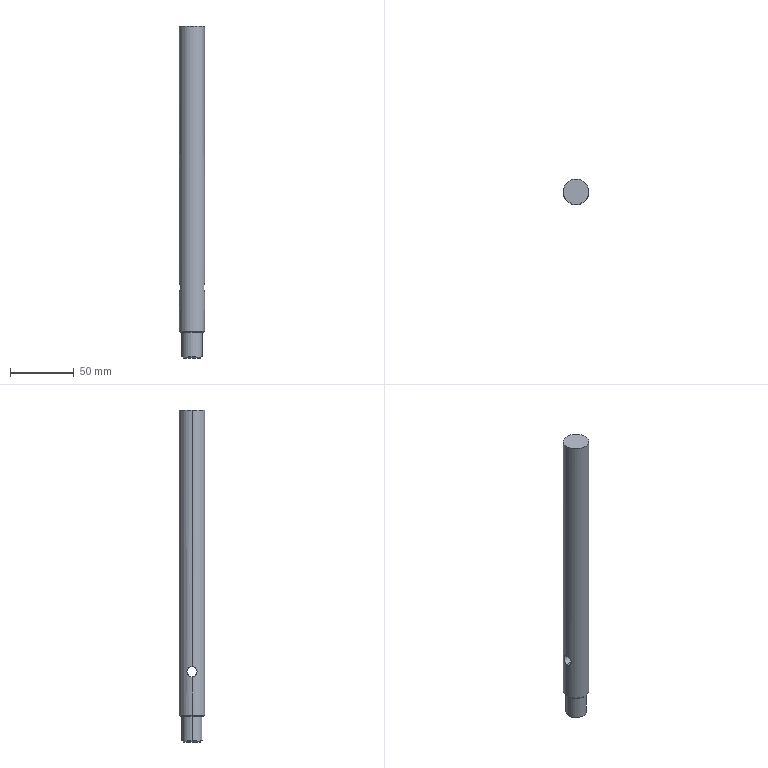Part | SolidWorks | features ICE 4, Chamfer 2, Revolution 1 | 1 solid | 13 faces | box 20 x 20 x 260 mm | volume 78380 mm3 | cylinder 6 | cone 4 | plane 3 | commonest cylinder face diameters 8 x2 16 x2 20 x2
STEP:
#1=CARTESIAN_POINT('',(-9.,0.,-170.));
#2=VERTEX_POINT('',#1);
#3=CARTESIAN_POINT('',(9.,0.,-170.));
#4=VERTEX_POINT('',#3);
#5=CARTESIAN_POINT('',(0.,0.,-170.));
#6=DIRECTION('',(0.,0.,-1.));
#7=DIRECTION('',(-1.,0.,0.));
#8=AXIS2_PLACEMENT_3D('',#5,#6,#7);
#9=CIRCLE('',#8,9.);
#10=EDGE_CURVE('',#2,#4,#9,.T.);
#11=ORIENTED_EDGE('',*,*,#10,.F.);
#12=CARTESIAN_POINT('',(-10.,0.,-169.));
#13=VERTEX_POINT('',#12);
#14=CARTESIAN_POINT('',(-9.,0.,-170.));
#15=DIRECTION('',(-0.7071,0.,0.7071));
#16=VECTOR('',#15,1000.);
#17=LINE('',#14,#16);
#18=EDGE_CURVE('',#2,#13,#17,.T.);
#19=ORIENTED_EDGE('',*,*,#18,.T.);
#20=CARTESIAN_POINT('',(10.,0.,-169.));
#21=VERTEX_POINT('',#20);
#22=CARTESIAN_POINT('',(0.,0.,-169.));
#23=DIRECTION('',(0.,0.,1.));
#24=DIRECTION('',(-1.,0.,0.));
#25=AXIS2_PLACEMENT_3D('',#22,#23,#24);
#26=CIRCLE('',#25,10.);
#27=EDGE_CURVE('',#21,#13,#26,.T.);
#28=ORIENTED_EDGE('',*,*,#27,.F.);
#29=CARTESIAN_POINT('',(9.,0.,-170.));
#30=DIRECTION('',(0.7071,0.,0.7071));
#31=VECTOR('',#30,1000.);
#32=LINE('',#29,#31);
#33=EDGE_CURVE('',#4,#21,#32,.T.);
#34=ORIENTED_EDGE('',*,*,#33,.F.);
#35=EDGE_LOOP('',(#11,#19,#28,#34));
#36=FACE_OUTER_BOUND('',#35,.T.);
#37=CARTESIAN_POINT('',(0.,0.,-170.));
#38=DIRECTION('',(0.,0.,1.));
#39=DIRECTION('',(1.,0.,0.));
#40=AXIS2_PLACEMENT_3D('',#37,#38,#39);
#41=CONICAL_SURFACE('',#40,9.,0.7854);
#42=ADVANCED_FACE('',(#36),#41,.T.);
#43=CARTESIAN_POINT('',(-7.,0.,-190.));
#44=VERTEX_POINT('',#43);
#45=CARTESIAN_POINT('',(7.,0.,-190.));
#46=VERTEX_POINT('',#45);
#47=CARTESIAN_POINT('',(0.,0.,-190.));
#48=DIRECTION('',(0.,0.,-1.));
#49=DIRECTION('',(-1.,0.,0.));
#50=AXIS2_PLACEMENT_3D('',#47,#48,#49);
#51=CIRCLE('',#50,7.);
#52=EDGE_CURVE('',#44,#46,#51,.T.);
#53=ORIENTED_EDGE('',*,*,#52,.F.);
#54=CARTESIAN_POINT('',(-8.,0.,-189.));
#55=VERTEX_POINT('',#54);
#56=CARTESIAN_POINT('',(-7.,0.,-190.));
#57=DIRECTION('',(-0.7071,0.,0.7071));
#58=VECTOR('',#57,1000.);
#59=LINE('',#56,#58);
#60=EDGE_CURVE('',#44,#55,#59,.T.);
#61=ORIENTED_EDGE('',*,*,#60,.T.);
#62=CARTESIAN_POINT('',(8.,0.,-189.));
#63=VERTEX_POINT('',#62);
#64=CARTESIAN_POINT('',(0.,0.,-189.));
#65=DIRECTION('',(0.,0.,1.));
#66=DIRECTION('',(-1.,0.,0.));
#67=AXIS2_PLACEMENT_3D('',#64,#65,#66);
#68=CIRCLE('',#67,8.);
#69=EDGE_CURVE('',#63,#55,#68,.T.);
#70=ORIENTED_EDGE('',*,*,#69,.F.);
#71=CARTESIAN_POINT('',(7.,0.,-190.));
#72=DIRECTION('',(0.7071,0.,0.7071));
#73=VECTOR('',#72,1000.);
#74=LINE('',#71,#73);
#75=EDGE_CURVE('',#46,#63,#74,.T.);
#76=ORIENTED_EDGE('',*,*,#75,.F.);
#77=EDGE_LOOP('',(#53,#61,#70,#76));
#78=FACE_OUTER_BOUND('',#77,.T.);
#79=CARTESIAN_POINT('',(0.,0.,-190.));
#80=DIRECTION('',(0.,0.,1.));
#81=DIRECTION('',(1.,0.,0.));
#82=AXIS2_PLACEMENT_3D('',#79,#80,#81);
#83=CONICAL_SURFACE('',#82,7.,0.7854);
#84=ADVANCED_FACE('',(#78),#83,.T.);
#85=ORIENTED_EDGE('',*,*,#69,.T.);
#86=CARTESIAN_POINT('',(-8.,0.,-170.));
#87=VERTEX_POINT('',#86);
#88=CARTESIAN_POINT('',(-8.,0.,-190.));
#89=DIRECTION('',(0.,0.,1.));
#90=VECTOR('',#89,1000.);
#91=LINE('',#88,#90);
#92=EDGE_CURVE('',#55,#87,#91,.T.);
#93=ORIENTED_EDGE('',*,*,#92,.T.);
#94=CARTESIAN_POINT('',(8.,0.,-170.));
#95=VERTEX_POINT('',#94);
#96=CARTESIAN_POINT('',(0.,0.,-170.));
#97=DIRECTION('',(0.,0.,-1.));
#98=DIRECTION('',(-1.,0.,0.));
#99=AXIS2_PLACEMENT_3D('',#96,#97,#98);
#100=CIRCLE('',#99,8.);
#101=EDGE_CURVE('',#87,#95,#100,.T.);
#102=ORIENTED_EDGE('',*,*,#101,.T.);
#103=CARTESIAN_POINT('',(8.,0.,-190.));
#104=DIRECTION('',(0.,0.,1.));
#105=VECTOR('',#104,1000.);
#106=LINE('',#103,#105);
#107=EDGE_CURVE('',#63,#95,#106,.T.);
#108=ORIENTED_EDGE('',*,*,#107,.F.);
#109=EDGE_LOOP('',(#85,#93,#102,#108));
#110=FACE_OUTER_BOUND('',#109,.T.);
#111=CARTESIAN_POINT('',(0.,0.,-190.));
#112=DIRECTION('',(0.,0.,1.));
#113=DIRECTION('',(1.,0.,0.));
#114=AXIS2_PLACEMENT_3D('',#111,#112,#113);
#115=CYLINDRICAL_SURFACE('',#114,8.);
#116=ADVANCED_FACE('',(#110),#115,.T.);
#117=CARTESIAN_POINT('',(10.,0.,-131.));
#118=VERTEX_POINT('',#117);
#119=CARTESIAN_POINT('',(10.,0.,-139.));
#120=VERTEX_POINT('',#119);
#121=CARTESIAN_POINT('',(10.,0.,-131.));
#122=CARTESIAN_POINT('',(10.,-0.2673,-131.));
#123=CARTESIAN_POINT('',(9.989,-0.5296,-131.027));
#124=CARTESIAN_POINT('',(9.949,-1.045,-131.13));
#125=CARTESIAN_POINT('',(9.918,-1.3,-131.208));
#126=CARTESIAN_POINT('',(9.843,-1.784,-131.41));
#127=CARTESIAN_POINT('',(9.798,-2.013,-131.533));
#128=CARTESIAN_POINT('',(9.699,-2.445,-131.824));
#129=CARTESIAN_POINT('',(9.645,-2.648,-131.991));
#130=CARTESIAN_POINT('',(9.537,-3.013,-132.356));
#131=CARTESIAN_POINT('',(9.483,-3.178,-132.556));
#132=CARTESIAN_POINT('',(9.38,-3.469,-132.991));
#133=CARTESIAN_POINT('',(9.333,-3.591,-133.22));
#134=CARTESIAN_POINT('',(9.254,-3.792,-133.7));
#135=CARTESIAN_POINT('',(9.221,-3.87,-133.954));
#136=CARTESIAN_POINT('',(9.177,-3.974,-134.472));
#137=CARTESIAN_POINT('',(9.165,-4.,-134.733));
#138=CARTESIAN_POINT('',(9.165,-4.,-135.262));
#139=CARTESIAN_POINT('',(9.177,-3.973,-135.53));
#140=CARTESIAN_POINT('',(9.221,-3.87,-136.045));
#141=CARTESIAN_POINT('',(9.253,-3.793,-136.297));
#142=CARTESIAN_POINT('',(9.334,-3.59,-136.784));
#143=CARTESIAN_POINT('',(9.381,-3.466,-137.013));
#144=CARTESIAN_POINT('',(9.483,-3.178,-137.443));
#145=CARTESIAN_POINT('',(9.538,-3.01,-137.646));
#146=CARTESIAN_POINT('',(9.646,-2.644,-138.012));
#147=CARTESIAN_POINT('',(9.699,-2.445,-138.176));
#148=CARTESIAN_POINT('',(9.798,-2.013,-138.466));
#149=CARTESIAN_POINT('',(9.843,-1.78,-138.592));
#150=CARTESIAN_POINT('',(9.918,-1.299,-138.792));
#151=CARTESIAN_POINT('',(9.948,-1.049,-138.869));
#152=CARTESIAN_POINT('',(9.99,-0.5273,-138.974));
#153=CARTESIAN_POINT('',(10.,-0.2633,-139.));
#154=CARTESIAN_POINT('',(10.,0.,-139.));
#155=B_SPLINE_CURVE_WITH_KNOTS('',3,(#121,#122,#123,#124,#125,#126,#127,#128,#129,#130,#131,#132,#133,#134,#135,#136,#137,#138,#139,#140,#141,#142,#143,#144,#145,#146,#147,#148,#149,#150,#151,#152,#153,#154),.UNSPECIFIED.,.F.,.F.,(4,2,2,2,2,2,2,2,2,2,2,2,2,2,2,2,4),(0.,0.00079,0.00158,0.00237,0.00316,0.00395,0.00474,0.00553,0.00632,0.00711,0.0079,0.00869,0.00948,0.01027,0.01106,0.01185,0.01264),.UNSPECIFIED.);
#156=EDGE_CURVE('',#118,#120,#155,.T.);
#157=ORIENTED_EDGE('',*,*,#156,.T.);
#158=CARTESIAN_POINT('',(-10.,0.,-139.));
#159=VERTEX_POINT('',#158);
#160=CARTESIAN_POINT('',(10.,0.,-139.));
#161=DIRECTION('',(-1.,0.,0.));
#162=VECTOR('',#161,1000.);
#163=LINE('',#160,#162);
#164=EDGE_CURVE('',#120,#159,#163,.T.);
#165=ORIENTED_EDGE('',*,*,#164,.T.);
#166=CARTESIAN_POINT('',(-10.,0.,-131.));
#167=VERTEX_POINT('',#166);
#168=CARTESIAN_POINT('',(-10.,0.,-139.));
#169=CARTESIAN_POINT('',(-10.,-0.2631,-139.));
#170=CARTESIAN_POINT('',(-9.989,-0.5298,-138.974));
#171=CARTESIAN_POINT('',(-9.948,-1.048,-138.869));
#172=CARTESIAN_POINT('',(-9.918,-1.299,-138.792));
#173=CARTESIAN_POINT('',(-9.843,-1.782,-138.591));
#174=CARTESIAN_POINT('',(-9.797,-2.015,-138.465));
#175=CARTESIAN_POINT('',(-9.699,-2.446,-138.176));
#176=CARTESIAN_POINT('',(-9.645,-2.646,-138.011));
#177=CARTESIAN_POINT('',(-9.537,-3.015,-137.642));
#178=CARTESIAN_POINT('',(-9.483,-3.179,-137.442));
#179=CARTESIAN_POINT('',(-9.381,-3.466,-137.013));
#180=CARTESIAN_POINT('',(-9.333,-3.592,-136.78));
#181=CARTESIAN_POINT('',(-9.253,-3.793,-136.297));
#182=CARTESIAN_POINT('',(-9.221,-3.869,-136.048));
#183=CARTESIAN_POINT('',(-9.177,-3.973,-135.532));
#184=CARTESIAN_POINT('',(-9.165,-4.,-135.264));
#185=CARTESIAN_POINT('',(-9.165,-4.,-134.737));
#186=CARTESIAN_POINT('',(-9.177,-3.974,-134.475));
#187=CARTESIAN_POINT('',(-9.221,-3.87,-133.954));
#188=CARTESIAN_POINT('',(-9.254,-3.792,-133.702));
#189=CARTESIAN_POINT('',(-9.333,-3.592,-133.22));
#190=CARTESIAN_POINT('',(-9.381,-3.467,-132.987));
#191=CARTESIAN_POINT('',(-9.483,-3.177,-132.556));
#192=CARTESIAN_POINT('',(-9.537,-3.013,-132.356));
#193=CARTESIAN_POINT('',(-9.645,-2.646,-131.989));
#194=CARTESIAN_POINT('',(-9.699,-2.443,-131.822));
#195=CARTESIAN_POINT('',(-9.798,-2.014,-131.534));
#196=CARTESIAN_POINT('',(-9.842,-1.785,-131.411));
#197=CARTESIAN_POINT('',(-9.918,-1.298,-131.207));
#198=CARTESIAN_POINT('',(-9.948,-1.046,-131.13));
#199=CARTESIAN_POINT('',(-9.989,-0.5323,-131.027));
#200=CARTESIAN_POINT('',(-10.,-0.2671,-131.));
#201=CARTESIAN_POINT('',(-10.,0.,-131.));
#202=B_SPLINE_CURVE_WITH_KNOTS('',3,(#168,#169,#170,#171,#172,#173,#174,#175,#176,#177,#178,#179,#180,#181,#182,#183,#184,#185,#186,#187,#188,#189,#190,#191,#192,#193,#194,#195,#196,#197,#198,#199,#200,#201),.UNSPECIFIED.,.F.,.F.,(4,2,2,2,2,2,2,2,2,2,2,2,2,2,2,2,4),(0.01264,0.01343,0.01422,0.01501,0.0158,0.01659,0.01738,0.01817,0.01896,0.01974,0.02053,0.02132,0.02211,0.0229,0.02369,0.02448,0.02527),.UNSPECIFIED.);
#203=EDGE_CURVE('',#159,#167,#202,.T.);
#204=ORIENTED_EDGE('',*,*,#203,.T.);
#205=CARTESIAN_POINT('',(10.,0.,-131.));
#206=DIRECTION('',(-1.,0.,0.));
#207=VECTOR('',#206,1000.);
#208=LINE('',#205,#207);
#209=EDGE_CURVE('',#118,#167,#208,.T.);
#210=ORIENTED_EDGE('',*,*,#209,.F.);
#211=EDGE_LOOP('',(#157,#165,#204,#210));
#212=FACE_OUTER_BOUND('',#211,.T.);
#213=CARTESIAN_POINT('',(10.,0.,-135.));
#214=DIRECTION('',(-1.,0.,0.));
#215=DIRECTION('',(0.,0.,1.));
#216=AXIS2_PLACEMENT_3D('',#213,#214,#215);
#217=CYLINDRICAL_SURFACE('',#216,4.);
#218=ADVANCED_FACE('',(#212),#217,.F.);
#219=ORIENTED_EDGE('',*,*,#27,.T.);
#220=CARTESIAN_POINT('',(-10.,0.,0.));
#221=DIRECTION('',(0.,0.,1.));
#222=VECTOR('',#221,1000.);
#223=LINE('',#220,#222);
#224=EDGE_CURVE('',#13,#159,#223,.T.);
#225=ORIENTED_EDGE('',*,*,#224,.T.);
#226=CARTESIAN_POINT('',(-10.,0.,-131.));
#227=CARTESIAN_POINT('',(-10.,0.2673,-131.));
#228=CARTESIAN_POINT('',(-9.989,0.5296,-131.027));
#229=CARTESIAN_POINT('',(-9.949,1.045,-131.13));
#230=CARTESIAN_POINT('',(-9.918,1.3,-131.208));
#231=CARTESIAN_POINT('',(-9.843,1.784,-131.41));
#232=CARTESIAN_POINT('',(-9.798,2.013,-131.533));
#233=CARTESIAN_POINT('',(-9.699,2.445,-131.824));
#234=CARTESIAN_POINT('',(-9.645,2.648,-131.991));
#235=CARTESIAN_POINT('',(-9.537,3.013,-132.356));
#236=CARTESIAN_POINT('',(-9.483,3.178,-132.556));
#237=CARTESIAN_POINT('',(-9.38,3.469,-132.991));
#238=CARTESIAN_POINT('',(-9.333,3.591,-133.22));
#239=CARTESIAN_POINT('',(-9.254,3.792,-133.7));
#240=CARTESIAN_POINT('',(-9.221,3.87,-133.954));
#241=CARTESIAN_POINT('',(-9.177,3.974,-134.472));
#242=CARTESIAN_POINT('',(-9.165,4.,-134.733));
#243=CARTESIAN_POINT('',(-9.165,4.,-135.262));
#244=CARTESIAN_POINT('',(-9.177,3.973,-135.53));
#245=CARTESIAN_POINT('',(-9.221,3.87,-136.045));
#246=CARTESIAN_POINT('',(-9.253,3.793,-136.297));
#247=CARTESIAN_POINT('',(-9.334,3.59,-136.784));
#248=CARTESIAN_POINT('',(-9.381,3.466,-137.013));
#249=CARTESIAN_POINT('',(-9.483,3.178,-137.443));
#250=CARTESIAN_POINT('',(-9.538,3.01,-137.646));
#251=CARTESIAN_POINT('',(-9.646,2.644,-138.012));
#252=CARTESIAN_POINT('',(-9.699,2.445,-138.176));
#253=CARTESIAN_POINT('',(-9.798,2.013,-138.466));
#254=CARTESIAN_POINT('',(-9.843,1.78,-138.592));
#255=CARTESIAN_POINT('',(-9.918,1.299,-138.792));
#256=CARTESIAN_POINT('',(-9.948,1.049,-138.869));
#257=CARTESIAN_POINT('',(-9.99,0.5273,-138.974));
#258=CARTESIAN_POINT('',(-10.,0.2633,-139.));
#259=CARTESIAN_POINT('',(-10.,0.,-139.));
#260=B_SPLINE_CURVE_WITH_KNOTS('',3,(#226,#227,#228,#229,#230,#231,#232,#233,#234,#235,#236,#237,#238,#239,#240,#241,#242,#243,#244,#245,#246,#247,#248,#249,#250,#251,#252,#253,#254,#255,#256,#257,#258,#259),.UNSPECIFIED.,.F.,.F.,(4,2,2,2,2,2,2,2,2,2,2,2,2,2,2,2,4),(0.,0.00079,0.00158,0.00237,0.00316,0.00395,0.00474,0.00553,0.00632,0.00711,0.0079,0.00869,0.00948,0.01027,0.01106,0.01185,0.01264),.UNSPECIFIED.);
#261=EDGE_CURVE('',#167,#159,#260,.T.);
#262=ORIENTED_EDGE('',*,*,#261,.F.);
#263=CARTESIAN_POINT('',(-10.,0.,70.));
#264=VERTEX_POINT('',#263);
#265=CARTESIAN_POINT('',(-10.,0.,0.));
#266=DIRECTION('',(0.,0.,1.));
#267=VECTOR('',#266,1000.);
#268=LINE('',#265,#267);
#269=EDGE_CURVE('',#167,#264,#268,.T.);
#270=ORIENTED_EDGE('',*,*,#269,.T.);
#271=CARTESIAN_POINT('',(10.,0.,70.));
#272=VERTEX_POINT('',#271);
#273=CARTESIAN_POINT('',(0.,0.,70.));
#274=DIRECTION('',(0.,0.,1.));
#275=DIRECTION('',(1.,0.,0.));
#276=AXIS2_PLACEMENT_3D('',#273,#274,#275);
#277=CIRCLE('',#276,10.);
#278=EDGE_CURVE('',#272,#264,#277,.T.);
#279=ORIENTED_EDGE('',*,*,#278,.F.);
#280=CARTESIAN_POINT('',(10.,0.,0.));
#281=DIRECTION('',(0.,0.,1.));
#282=VECTOR('',#281,1000.);
#283=LINE('',#280,#282);
#284=EDGE_CURVE('',#118,#272,#283,.T.);
#285=ORIENTED_EDGE('',*,*,#284,.F.);
#286=CARTESIAN_POINT('',(10.,0.,-139.));
#287=CARTESIAN_POINT('',(10.,0.2631,-139.));
#288=CARTESIAN_POINT('',(9.989,0.5298,-138.974));
#289=CARTESIAN_POINT('',(9.948,1.048,-138.869));
#290=CARTESIAN_POINT('',(9.918,1.299,-138.792));
#291=CARTESIAN_POINT('',(9.843,1.782,-138.591));
#292=CARTESIAN_POINT('',(9.797,2.015,-138.465));
#293=CARTESIAN_POINT('',(9.699,2.446,-138.176));
#294=CARTESIAN_POINT('',(9.645,2.646,-138.011));
#295=CARTESIAN_POINT('',(9.537,3.015,-137.642));
#296=CARTESIAN_POINT('',(9.483,3.179,-137.442));
#297=CARTESIAN_POINT('',(9.381,3.466,-137.013));
#298=CARTESIAN_POINT('',(9.333,3.592,-136.78));
#299=CARTESIAN_POINT('',(9.253,3.793,-136.297));
#300=CARTESIAN_POINT('',(9.221,3.869,-136.048));
#301=CARTESIAN_POINT('',(9.177,3.973,-135.532));
#302=CARTESIAN_POINT('',(9.165,4.,-135.264));
#303=CARTESIAN_POINT('',(9.165,4.,-134.737));
#304=CARTESIAN_POINT('',(9.177,3.974,-134.475));
#305=CARTESIAN_POINT('',(9.221,3.87,-133.954));
#306=CARTESIAN_POINT('',(9.254,3.792,-133.702));
#307=CARTESIAN_POINT('',(9.333,3.592,-133.22));
#308=CARTESIAN_POINT('',(9.381,3.467,-132.987));
#309=CARTESIAN_POINT('',(9.483,3.177,-132.556));
#310=CARTESIAN_POINT('',(9.537,3.013,-132.356));
#311=CARTESIAN_POINT('',(9.645,2.646,-131.989));
#312=CARTESIAN_POINT('',(9.699,2.443,-131.822));
#313=CARTESIAN_POINT('',(9.798,2.014,-131.534));
#314=CARTESIAN_POINT('',(9.842,1.785,-131.411));
#315=CARTESIAN_POINT('',(9.918,1.298,-131.207));
#316=CARTESIAN_POINT('',(9.948,1.046,-131.13));
#317=CARTESIAN_POINT('',(9.989,0.5323,-131.027));
#318=CARTESIAN_POINT('',(10.,0.2671,-131.));
#319=CARTESIAN_POINT('',(10.,0.,-131.));
#320=B_SPLINE_CURVE_WITH_KNOTS('',3,(#286,#287,#288,#289,#290,#291,#292,#293,#294,#295,#296,#297,#298,#299,#300,#301,#302,#303,#304,#305,#306,#307,#308,#309,#310,#311,#312,#313,#314,#315,#316,#317,#318,#319),.UNSPECIFIED.,.F.,.F.,(4,2,2,2,2,2,2,2,2,2,2,2,2,2,2,2,4),(0.01264,0.01343,0.01422,0.01501,0.0158,0.01659,0.01738,0.01817,0.01896,0.01974,0.02053,0.02132,0.02211,0.0229,0.02369,0.02448,0.02527),.UNSPECIFIED.);
#321=EDGE_CURVE('',#120,#118,#320,.T.);
#322=ORIENTED_EDGE('',*,*,#321,.F.);
#323=CARTESIAN_POINT('',(10.,0.,0.));
#324=DIRECTION('',(0.,0.,1.));
#325=VECTOR('',#324,1000.);
#326=LINE('',#323,#325);
#327=EDGE_CURVE('',#21,#120,#326,.T.);
#328=ORIENTED_EDGE('',*,*,#327,.F.);
#329=EDGE_LOOP('',(#219,#225,#262,#270,#279,#285,#322,#328));
#330=FACE_OUTER_BOUND('',#329,.T.);
#331=CARTESIAN_POINT('',(0.,0.,0.));
#332=DIRECTION('',(0.,0.,1.));
#333=DIRECTION('',(1.,0.,0.));
#334=AXIS2_PLACEMENT_3D('',#331,#332,#333);
#335=CYLINDRICAL_SURFACE('',#334,10.);
#336=ADVANCED_FACE('',(#330),#335,.T.);
#337=ORIENTED_EDGE('',*,*,#224,.F.);
#338=CARTESIAN_POINT('',(0.,0.,-169.));
#339=DIRECTION('',(0.,0.,1.));
#340=DIRECTION('',(-1.,0.,0.));
#341=AXIS2_PLACEMENT_3D('',#338,#339,#340);
#342=CIRCLE('',#341,10.);
#343=EDGE_CURVE('',#13,#21,#342,.T.);
#344=ORIENTED_EDGE('',*,*,#343,.T.);
#345=ORIENTED_EDGE('',*,*,#327,.T.);
#346=ORIENTED_EDGE('',*,*,#156,.F.);
#347=ORIENTED_EDGE('',*,*,#284,.T.);
#348=CARTESIAN_POINT('',(0.,0.,70.));
#349=DIRECTION('',(0.,0.,1.));
#350=DIRECTION('',(1.,0.,0.));
#351=AXIS2_PLACEMENT_3D('',#348,#349,#350);
#352=CIRCLE('',#351,10.);
#353=EDGE_CURVE('',#264,#272,#352,.T.);
#354=ORIENTED_EDGE('',*,*,#353,.F.);
#355=ORIENTED_EDGE('',*,*,#269,.F.);
#356=ORIENTED_EDGE('',*,*,#203,.F.);
#357=EDGE_LOOP('',(#337,#344,#345,#346,#347,#354,#355,#356));
#358=FACE_OUTER_BOUND('',#357,.T.);
#359=CARTESIAN_POINT('',(0.,0.,0.));
#360=DIRECTION('',(0.,0.,1.));
#361=DIRECTION('',(1.,0.,0.));
#362=AXIS2_PLACEMENT_3D('',#359,#360,#361);
#363=CYLINDRICAL_SURFACE('',#362,10.);
#364=ADVANCED_FACE('',(#358),#363,.T.);
#365=ORIENTED_EDGE('',*,*,#164,.F.);
#366=ORIENTED_EDGE('',*,*,#321,.T.);
#367=ORIENTED_EDGE('',*,*,#209,.T.);
#368=ORIENTED_EDGE('',*,*,#261,.T.);
#369=EDGE_LOOP('',(#365,#366,#367,#368));
#370=FACE_OUTER_BOUND('',#369,.T.);
#371=CARTESIAN_POINT('',(10.,0.,-135.));
#372=DIRECTION('',(-1.,0.,0.));
#373=DIRECTION('',(0.,0.,1.));
#374=AXIS2_PLACEMENT_3D('',#371,#372,#373);
#375=CYLINDRICAL_SURFACE('',#374,4.);
#376=ADVANCED_FACE('',(#370),#375,.F.);
#377=ORIENTED_EDGE('',*,*,#278,.T.);
#378=ORIENTED_EDGE('',*,*,#353,.T.);
#379=EDGE_LOOP('',(#377,#378));
#380=FACE_OUTER_BOUND('',#379,.T.);
#381=CARTESIAN_POINT('',(0.,0.,70.));
#382=DIRECTION('',(0.,0.,1.));
#383=DIRECTION('',(1.,0.,0.));
#384=AXIS2_PLACEMENT_3D('',#381,#382,#383);
#385=PLANE('',#384);
#386=ADVANCED_FACE('',(#380),#385,.T.);
#387=CARTESIAN_POINT('',(0.,0.,-170.));
#388=DIRECTION('',(0.,0.,-1.));
#389=DIRECTION('',(-1.,0.,0.));
#390=AXIS2_PLACEMENT_3D('',#387,#388,#389);
#391=CIRCLE('',#390,9.);
#392=EDGE_CURVE('',#4,#2,#391,.T.);
#393=ORIENTED_EDGE('',*,*,#392,.T.);
#394=ORIENTED_EDGE('',*,*,#10,.T.);
#395=EDGE_LOOP('',(#393,#394));
#396=FACE_OUTER_BOUND('',#395,.T.);
#397=CARTESIAN_POINT('',(0.,0.,-170.));
#398=DIRECTION('',(0.,0.,-1.));
#399=DIRECTION('',(-1.,0.,0.));
#400=AXIS2_PLACEMENT_3D('',#397,#398,#399);
#401=CIRCLE('',#400,8.);
#402=EDGE_CURVE('',#95,#87,#401,.T.);
#403=ORIENTED_EDGE('',*,*,#402,.F.);
#404=ORIENTED_EDGE('',*,*,#101,.F.);
#405=EDGE_LOOP('',(#403,#404));
#406=FACE_BOUND('',#405,.T.);
#407=CARTESIAN_POINT('',(0.,0.,-170.));
#408=DIRECTION('',(0.,0.,-1.));
#409=DIRECTION('',(-1.,0.,0.));
#410=AXIS2_PLACEMENT_3D('',#407,#408,#409);
#411=PLANE('',#410);
#412=ADVANCED_FACE('',(#396,#406),#411,.T.);
#413=ORIENTED_EDGE('',*,*,#92,.F.);
#414=CARTESIAN_POINT('',(0.,0.,-189.));
#415=DIRECTION('',(0.,0.,1.));
#416=DIRECTION('',(-1.,0.,0.));
#417=AXIS2_PLACEMENT_3D('',#414,#415,#416);
#418=CIRCLE('',#417,8.);
#419=EDGE_CURVE('',#55,#63,#418,.T.);
#420=ORIENTED_EDGE('',*,*,#419,.T.);
#421=ORIENTED_EDGE('',*,*,#107,.T.);
#422=ORIENTED_EDGE('',*,*,#402,.T.);
#423=EDGE_LOOP('',(#413,#420,#421,#422));
#424=FACE_OUTER_BOUND('',#423,.T.);
#425=CARTESIAN_POINT('',(0.,0.,-190.));
#426=DIRECTION('',(0.,0.,1.));
#427=DIRECTION('',(1.,0.,0.));
#428=AXIS2_PLACEMENT_3D('',#425,#426,#427);
#429=CYLINDRICAL_SURFACE('',#428,8.);
#430=ADVANCED_FACE('',(#424),#429,.T.);
#431=CARTESIAN_POINT('',(0.,0.,-190.));
#432=DIRECTION('',(0.,0.,-1.));
#433=DIRECTION('',(-1.,0.,0.));
#434=AXIS2_PLACEMENT_3D('',#431,#432,#433);
#435=CIRCLE('',#434,7.);
#436=EDGE_CURVE('',#46,#44,#435,.T.);
#437=ORIENTED_EDGE('',*,*,#436,.T.);
#438=ORIENTED_EDGE('',*,*,#52,.T.);
#439=EDGE_LOOP('',(#437,#438));
#440=FACE_OUTER_BOUND('',#439,.T.);
#441=CARTESIAN_POINT('',(0.,0.,-190.));
#442=DIRECTION('',(0.,0.,-1.));
#443=DIRECTION('',(-1.,0.,0.));
#444=AXIS2_PLACEMENT_3D('',#441,#442,#443);
#445=PLANE('',#444);
#446=ADVANCED_FACE('',(#440),#445,.T.);
#447=ORIENTED_EDGE('',*,*,#60,.F.);
#448=ORIENTED_EDGE('',*,*,#436,.F.);
#449=ORIENTED_EDGE('',*,*,#75,.T.);
#450=ORIENTED_EDGE('',*,*,#419,.F.);
#451=EDGE_LOOP('',(#447,#448,#449,#450));
#452=FACE_OUTER_BOUND('',#451,.T.);
#453=CARTESIAN_POINT('',(0.,0.,-190.));
#454=DIRECTION('',(0.,0.,1.));
#455=DIRECTION('',(1.,0.,0.));
#456=AXIS2_PLACEMENT_3D('',#453,#454,#455);
#457=CONICAL_SURFACE('',#456,7.,0.7854);
#458=ADVANCED_FACE('',(#452),#457,.T.);
#459=ORIENTED_EDGE('',*,*,#18,.F.);
#460=ORIENTED_EDGE('',*,*,#392,.F.);
#461=ORIENTED_EDGE('',*,*,#33,.T.);
#462=ORIENTED_EDGE('',*,*,#343,.F.);
#463=EDGE_LOOP('',(#459,#460,#461,#462));
#464=FACE_OUTER_BOUND('',#463,.T.);
#465=CARTESIAN_POINT('',(0.,0.,-170.));
#466=DIRECTION('',(0.,0.,1.));
#467=DIRECTION('',(1.,0.,0.));
#468=AXIS2_PLACEMENT_3D('',#465,#466,#467);
#469=CONICAL_SURFACE('',#468,9.,0.7854);
#470=ADVANCED_FACE('',(#464),#469,.T.);
#471=CLOSED_SHELL('',(#42,#84,#116,#218,#336,#364,#376,#386,#412,#430,#446,#458,#470));
#472=MANIFOLD_SOLID_BREP('',#471);
#473=CARTESIAN_POINT('',(0.,0.,0.));
#474=DIRECTION('',(0.,0.,1.));
#475=DIRECTION('',(1.,0.,0.));
#476=AXIS2_PLACEMENT_3D('',#473,#474,#475);
#477=(LENGTH_UNIT()NAMED_UNIT(*)SI_UNIT(.MILLI.,.METRE.));
#478=UNCERTAINTY_MEASURE_WITH_UNIT(LENGTH_MEASURE(0.00001),#477,'','');
#479=(NAMED_UNIT(*)PLANE_ANGLE_UNIT()SI_UNIT($,.RADIAN.));
#480=(NAMED_UNIT(*)SI_UNIT($,.STERADIAN.)SOLID_ANGLE_UNIT());
#481=(GEOMETRIC_REPRESENTATION_CONTEXT(3)GLOBAL_UNCERTAINTY_ASSIGNED_CONTEXT((#478))GLOBAL_UNIT_ASSIGNED_CONTEXT((#477,#479,#480))REPRESENTATION_CONTEXT('',''));
#482=ADVANCED_BREP_SHAPE_REPRESENTATION('',(#472,#476),#481);